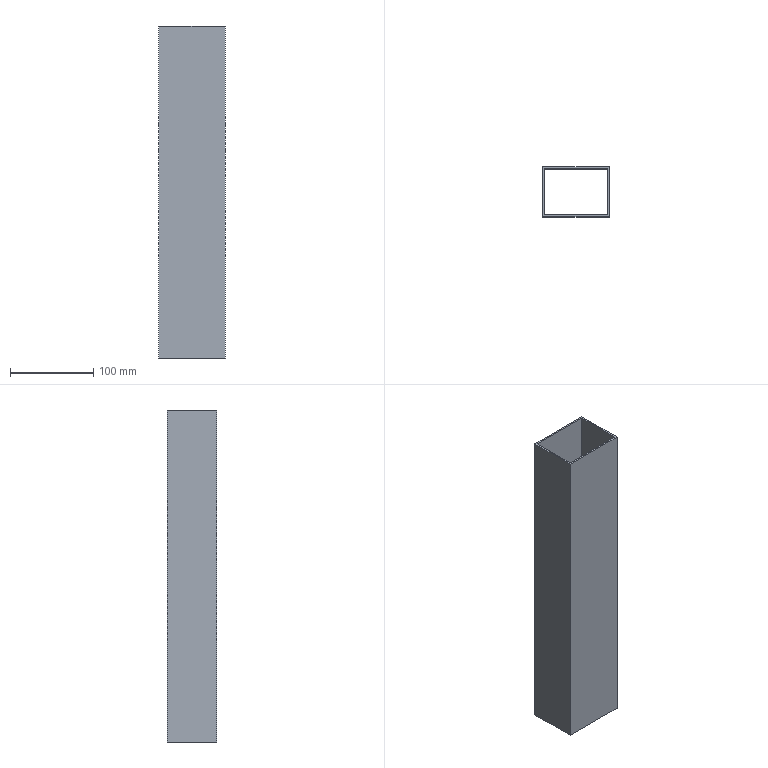Part | STEP file | Guide wheel mechanism revised.sldasm-Part-176 | 1 solid | 10 faces | box 80 x 60 x 400 mm | volume 217600 mm3 | plane 10
STEP:
#1=CARTESIAN_POINT('',(440.,1428.01,-200.));
#2=VERTEX_POINT('',#1);
#3=CARTESIAN_POINT('',(360.,1428.01,-200.));
#4=VERTEX_POINT('',#3);
#5=CARTESIAN_POINT('',(360.,1428.01,-200.));
#6=DIRECTION('',(-1.,0.,0.));
#7=VECTOR('',#6,1000.);
#8=LINE('',#5,#7);
#9=EDGE_CURVE('',#2,#4,#8,.T.);
#10=ORIENTED_EDGE('',*,*,#9,.F.);
#11=CARTESIAN_POINT('',(440.,1428.01,200.));
#12=VERTEX_POINT('',#11);
#13=CARTESIAN_POINT('',(440.,1428.01,-300.));
#14=DIRECTION('',(0.,0.,1.));
#15=VECTOR('',#14,1000.);
#16=LINE('',#13,#15);
#17=EDGE_CURVE('',#2,#12,#16,.T.);
#18=ORIENTED_EDGE('',*,*,#17,.T.);
#19=CARTESIAN_POINT('',(360.,1428.01,200.));
#20=VERTEX_POINT('',#19);
#21=CARTESIAN_POINT('',(360.,1428.01,200.));
#22=DIRECTION('',(-1.,0.,0.));
#23=VECTOR('',#22,1000.);
#24=LINE('',#21,#23);
#25=EDGE_CURVE('',#12,#20,#24,.T.);
#26=ORIENTED_EDGE('',*,*,#25,.T.);
#27=CARTESIAN_POINT('',(360.,1428.01,-300.));
#28=DIRECTION('',(0.,0.,1.));
#29=VECTOR('',#28,1000.);
#30=LINE('',#27,#29);
#31=EDGE_CURVE('',#4,#20,#30,.T.);
#32=ORIENTED_EDGE('',*,*,#31,.F.);
#33=EDGE_LOOP('',(#10,#18,#26,#32));
#34=FACE_OUTER_BOUND('',#33,.T.);
#35=CARTESIAN_POINT('',(360.,1428.01,-300.));
#36=DIRECTION('',(0.,1.,0.));
#37=DIRECTION('',(0.,0.,1.));
#38=AXIS2_PLACEMENT_3D('',#35,#36,#37);
#39=PLANE('',#38);
#40=ADVANCED_FACE('',(#34),#39,.F.);
#41=CARTESIAN_POINT('',(440.,1488.01,-200.));
#42=VERTEX_POINT('',#41);
#43=CARTESIAN_POINT('',(440.,1428.01,-200.));
#44=DIRECTION('',(0.,-1.,0.));
#45=VECTOR('',#44,1000.);
#46=LINE('',#43,#45);
#47=EDGE_CURVE('',#42,#2,#46,.T.);
#48=ORIENTED_EDGE('',*,*,#47,.F.);
#49=CARTESIAN_POINT('',(440.,1488.01,200.));
#50=VERTEX_POINT('',#49);
#51=CARTESIAN_POINT('',(440.,1488.01,-300.));
#52=DIRECTION('',(0.,0.,1.));
#53=VECTOR('',#52,1000.);
#54=LINE('',#51,#53);
#55=EDGE_CURVE('',#42,#50,#54,.T.);
#56=ORIENTED_EDGE('',*,*,#55,.T.);
#57=CARTESIAN_POINT('',(440.,1428.01,200.));
#58=DIRECTION('',(0.,-1.,0.));
#59=VECTOR('',#58,1000.);
#60=LINE('',#57,#59);
#61=EDGE_CURVE('',#50,#12,#60,.T.);
#62=ORIENTED_EDGE('',*,*,#61,.T.);
#63=ORIENTED_EDGE('',*,*,#17,.F.);
#64=EDGE_LOOP('',(#48,#56,#62,#63));
#65=FACE_OUTER_BOUND('',#64,.T.);
#66=CARTESIAN_POINT('',(440.,1428.01,-300.));
#67=DIRECTION('',(-1.,0.,0.));
#68=DIRECTION('',(0.,0.,1.));
#69=AXIS2_PLACEMENT_3D('',#66,#67,#68);
#70=PLANE('',#69);
#71=ADVANCED_FACE('',(#65),#70,.F.);
#72=CARTESIAN_POINT('',(360.,1488.01,-200.));
#73=VERTEX_POINT('',#72);
#74=CARTESIAN_POINT('',(360.,1488.01,-200.));
#75=DIRECTION('',(1.,0.,0.));
#76=VECTOR('',#75,1000.);
#77=LINE('',#74,#76);
#78=EDGE_CURVE('',#73,#42,#77,.T.);
#79=ORIENTED_EDGE('',*,*,#78,.F.);
#80=CARTESIAN_POINT('',(360.,1488.01,200.));
#81=VERTEX_POINT('',#80);
#82=CARTESIAN_POINT('',(360.,1488.01,-300.));
#83=DIRECTION('',(0.,0.,1.));
#84=VECTOR('',#83,1000.);
#85=LINE('',#82,#84);
#86=EDGE_CURVE('',#73,#81,#85,.T.);
#87=ORIENTED_EDGE('',*,*,#86,.T.);
#88=CARTESIAN_POINT('',(360.,1488.01,200.));
#89=DIRECTION('',(1.,0.,0.));
#90=VECTOR('',#89,1000.);
#91=LINE('',#88,#90);
#92=EDGE_CURVE('',#81,#50,#91,.T.);
#93=ORIENTED_EDGE('',*,*,#92,.T.);
#94=ORIENTED_EDGE('',*,*,#55,.F.);
#95=EDGE_LOOP('',(#79,#87,#93,#94));
#96=FACE_OUTER_BOUND('',#95,.T.);
#97=CARTESIAN_POINT('',(360.,1488.01,-300.));
#98=DIRECTION('',(0.,-1.,0.));
#99=DIRECTION('',(0.,0.,-1.));
#100=AXIS2_PLACEMENT_3D('',#97,#98,#99);
#101=PLANE('',#100);
#102=ADVANCED_FACE('',(#96),#101,.F.);
#103=CARTESIAN_POINT('',(360.,1428.01,-200.));
#104=DIRECTION('',(0.,1.,0.));
#105=VECTOR('',#104,1000.);
#106=LINE('',#103,#105);
#107=EDGE_CURVE('',#4,#73,#106,.T.);
#108=ORIENTED_EDGE('',*,*,#107,.F.);
#109=ORIENTED_EDGE('',*,*,#31,.T.);
#110=CARTESIAN_POINT('',(360.,1428.01,200.));
#111=DIRECTION('',(0.,1.,0.));
#112=VECTOR('',#111,1000.);
#113=LINE('',#110,#112);
#114=EDGE_CURVE('',#20,#81,#113,.T.);
#115=ORIENTED_EDGE('',*,*,#114,.T.);
#116=ORIENTED_EDGE('',*,*,#86,.F.);
#117=EDGE_LOOP('',(#108,#109,#115,#116));
#118=FACE_OUTER_BOUND('',#117,.T.);
#119=CARTESIAN_POINT('',(360.,1428.01,-300.));
#120=DIRECTION('',(1.,0.,0.));
#121=DIRECTION('',(0.,0.,-1.));
#122=AXIS2_PLACEMENT_3D('',#119,#120,#121);
#123=PLANE('',#122);
#124=ADVANCED_FACE('',(#118),#123,.F.);
#125=ORIENTED_EDGE('',*,*,#114,.F.);
#126=ORIENTED_EDGE('',*,*,#25,.F.);
#127=ORIENTED_EDGE('',*,*,#61,.F.);
#128=ORIENTED_EDGE('',*,*,#92,.F.);
#129=EDGE_LOOP('',(#125,#126,#127,#128));
#130=FACE_OUTER_BOUND('',#129,.T.);
#131=CARTESIAN_POINT('',(362.,1430.01,200.));
#132=VERTEX_POINT('',#131);
#133=CARTESIAN_POINT('',(362.,1486.01,200.));
#134=VERTEX_POINT('',#133);
#135=CARTESIAN_POINT('',(362.,1430.01,200.));
#136=DIRECTION('',(0.,1.,0.));
#137=VECTOR('',#136,1000.);
#138=LINE('',#135,#137);
#139=EDGE_CURVE('',#132,#134,#138,.T.);
#140=ORIENTED_EDGE('',*,*,#139,.T.);
#141=CARTESIAN_POINT('',(438.,1486.01,200.));
#142=VERTEX_POINT('',#141);
#143=CARTESIAN_POINT('',(362.,1486.01,200.));
#144=DIRECTION('',(1.,0.,0.));
#145=VECTOR('',#144,1000.);
#146=LINE('',#143,#145);
#147=EDGE_CURVE('',#134,#142,#146,.T.);
#148=ORIENTED_EDGE('',*,*,#147,.T.);
#149=CARTESIAN_POINT('',(438.,1430.01,200.));
#150=VERTEX_POINT('',#149);
#151=CARTESIAN_POINT('',(438.,1430.01,200.));
#152=DIRECTION('',(0.,-1.,0.));
#153=VECTOR('',#152,1000.);
#154=LINE('',#151,#153);
#155=EDGE_CURVE('',#142,#150,#154,.T.);
#156=ORIENTED_EDGE('',*,*,#155,.T.);
#157=CARTESIAN_POINT('',(362.,1430.01,200.));
#158=DIRECTION('',(-1.,0.,0.));
#159=VECTOR('',#158,1000.);
#160=LINE('',#157,#159);
#161=EDGE_CURVE('',#150,#132,#160,.T.);
#162=ORIENTED_EDGE('',*,*,#161,.T.);
#163=EDGE_LOOP('',(#140,#148,#156,#162));
#164=FACE_BOUND('',#163,.T.);
#165=CARTESIAN_POINT('',(0.,0.,200.));
#166=DIRECTION('',(0.,0.,-1.));
#167=DIRECTION('',(-1.,0.,0.));
#168=AXIS2_PLACEMENT_3D('',#165,#166,#167);
#169=PLANE('',#168);
#170=ADVANCED_FACE('',(#130,#164),#169,.F.);
#171=CARTESIAN_POINT('',(438.,1430.01,-200.));
#172=VERTEX_POINT('',#171);
#173=CARTESIAN_POINT('',(438.,1430.01,-300.));
#174=DIRECTION('',(0.,0.,1.));
#175=VECTOR('',#174,1000.);
#176=LINE('',#173,#175);
#177=EDGE_CURVE('',#172,#150,#176,.T.);
#178=ORIENTED_EDGE('',*,*,#177,.F.);
#179=CARTESIAN_POINT('',(362.,1430.01,-200.));
#180=VERTEX_POINT('',#179);
#181=CARTESIAN_POINT('',(362.,1430.01,-200.));
#182=DIRECTION('',(-1.,0.,0.));
#183=VECTOR('',#182,1000.);
#184=LINE('',#181,#183);
#185=EDGE_CURVE('',#172,#180,#184,.T.);
#186=ORIENTED_EDGE('',*,*,#185,.T.);
#187=CARTESIAN_POINT('',(362.,1430.01,-300.));
#188=DIRECTION('',(0.,0.,1.));
#189=VECTOR('',#188,1000.);
#190=LINE('',#187,#189);
#191=EDGE_CURVE('',#180,#132,#190,.T.);
#192=ORIENTED_EDGE('',*,*,#191,.T.);
#193=ORIENTED_EDGE('',*,*,#161,.F.);
#194=EDGE_LOOP('',(#178,#186,#192,#193));
#195=FACE_OUTER_BOUND('',#194,.T.);
#196=CARTESIAN_POINT('',(362.,1430.01,-300.));
#197=DIRECTION('',(0.,1.,0.));
#198=DIRECTION('',(0.,0.,1.));
#199=AXIS2_PLACEMENT_3D('',#196,#197,#198);
#200=PLANE('',#199);
#201=ADVANCED_FACE('',(#195),#200,.T.);
#202=CARTESIAN_POINT('',(438.,1486.01,-200.));
#203=VERTEX_POINT('',#202);
#204=CARTESIAN_POINT('',(438.,1486.01,-300.));
#205=DIRECTION('',(0.,0.,1.));
#206=VECTOR('',#205,1000.);
#207=LINE('',#204,#206);
#208=EDGE_CURVE('',#203,#142,#207,.T.);
#209=ORIENTED_EDGE('',*,*,#208,.F.);
#210=CARTESIAN_POINT('',(438.,1430.01,-200.));
#211=DIRECTION('',(0.,-1.,0.));
#212=VECTOR('',#211,1000.);
#213=LINE('',#210,#212);
#214=EDGE_CURVE('',#203,#172,#213,.T.);
#215=ORIENTED_EDGE('',*,*,#214,.T.);
#216=ORIENTED_EDGE('',*,*,#177,.T.);
#217=ORIENTED_EDGE('',*,*,#155,.F.);
#218=EDGE_LOOP('',(#209,#215,#216,#217));
#219=FACE_OUTER_BOUND('',#218,.T.);
#220=CARTESIAN_POINT('',(438.,1430.01,-300.));
#221=DIRECTION('',(-1.,0.,0.));
#222=DIRECTION('',(0.,0.,1.));
#223=AXIS2_PLACEMENT_3D('',#220,#221,#222);
#224=PLANE('',#223);
#225=ADVANCED_FACE('',(#219),#224,.T.);
#226=CARTESIAN_POINT('',(362.,1486.01,-200.));
#227=VERTEX_POINT('',#226);
#228=CARTESIAN_POINT('',(362.,1486.01,-300.));
#229=DIRECTION('',(0.,0.,1.));
#230=VECTOR('',#229,1000.);
#231=LINE('',#228,#230);
#232=EDGE_CURVE('',#227,#134,#231,.T.);
#233=ORIENTED_EDGE('',*,*,#232,.F.);
#234=CARTESIAN_POINT('',(362.,1486.01,-200.));
#235=DIRECTION('',(1.,0.,0.));
#236=VECTOR('',#235,1000.);
#237=LINE('',#234,#236);
#238=EDGE_CURVE('',#227,#203,#237,.T.);
#239=ORIENTED_EDGE('',*,*,#238,.T.);
#240=ORIENTED_EDGE('',*,*,#208,.T.);
#241=ORIENTED_EDGE('',*,*,#147,.F.);
#242=EDGE_LOOP('',(#233,#239,#240,#241));
#243=FACE_OUTER_BOUND('',#242,.T.);
#244=CARTESIAN_POINT('',(362.,1486.01,-300.));
#245=DIRECTION('',(0.,-1.,0.));
#246=DIRECTION('',(0.,0.,-1.));
#247=AXIS2_PLACEMENT_3D('',#244,#245,#246);
#248=PLANE('',#247);
#249=ADVANCED_FACE('',(#243),#248,.T.);
#250=ORIENTED_EDGE('',*,*,#191,.F.);
#251=CARTESIAN_POINT('',(362.,1430.01,-200.));
#252=DIRECTION('',(0.,1.,0.));
#253=VECTOR('',#252,1000.);
#254=LINE('',#251,#253);
#255=EDGE_CURVE('',#180,#227,#254,.T.);
#256=ORIENTED_EDGE('',*,*,#255,.T.);
#257=ORIENTED_EDGE('',*,*,#232,.T.);
#258=ORIENTED_EDGE('',*,*,#139,.F.);
#259=EDGE_LOOP('',(#250,#256,#257,#258));
#260=FACE_OUTER_BOUND('',#259,.T.);
#261=CARTESIAN_POINT('',(362.,1430.01,-300.));
#262=DIRECTION('',(1.,0.,0.));
#263=DIRECTION('',(0.,0.,-1.));
#264=AXIS2_PLACEMENT_3D('',#261,#262,#263);
#265=PLANE('',#264);
#266=ADVANCED_FACE('',(#260),#265,.T.);
#267=ORIENTED_EDGE('',*,*,#255,.F.);
#268=ORIENTED_EDGE('',*,*,#185,.F.);
#269=ORIENTED_EDGE('',*,*,#214,.F.);
#270=ORIENTED_EDGE('',*,*,#238,.F.);
#271=EDGE_LOOP('',(#267,#268,#269,#270));
#272=FACE_BOUND('',#271,.T.);
#273=ORIENTED_EDGE('',*,*,#9,.T.);
#274=ORIENTED_EDGE('',*,*,#107,.T.);
#275=ORIENTED_EDGE('',*,*,#78,.T.);
#276=ORIENTED_EDGE('',*,*,#47,.T.);
#277=EDGE_LOOP('',(#273,#274,#275,#276));
#278=FACE_OUTER_BOUND('',#277,.T.);
#279=CARTESIAN_POINT('',(-360.,1970.,-200.));
#280=DIRECTION('',(0.,0.,-1.));
#281=DIRECTION('',(-1.,0.,0.));
#282=AXIS2_PLACEMENT_3D('',#279,#280,#281);
#283=PLANE('',#282);
#284=ADVANCED_FACE('',(#272,#278),#283,.T.);
#285=CLOSED_SHELL('',(#40,#71,#102,#124,#170,#201,#225,#249,#266,#284));
#286=MANIFOLD_SOLID_BREP('',#285);
#287=CARTESIAN_POINT('',(0.,0.,0.));
#288=DIRECTION('',(0.,0.,1.));
#289=DIRECTION('',(1.,0.,0.));
#290=AXIS2_PLACEMENT_3D('',#287,#288,#289);
#291=(LENGTH_UNIT()NAMED_UNIT(*)SI_UNIT(.MILLI.,.METRE.));
#292=UNCERTAINTY_MEASURE_WITH_UNIT(LENGTH_MEASURE(0.00001),#291,'','');
#293=(NAMED_UNIT(*)PLANE_ANGLE_UNIT()SI_UNIT($,.RADIAN.));
#294=(NAMED_UNIT(*)SI_UNIT($,.STERADIAN.)SOLID_ANGLE_UNIT());
#295=(GEOMETRIC_REPRESENTATION_CONTEXT(3)GLOBAL_UNCERTAINTY_ASSIGNED_CONTEXT((#292))GLOBAL_UNIT_ASSIGNED_CONTEXT((#291,#293,#294))REPRESENTATION_CONTEXT('',''));
#296=ADVANCED_BREP_SHAPE_REPRESENTATION('',(#286,#290),#295);